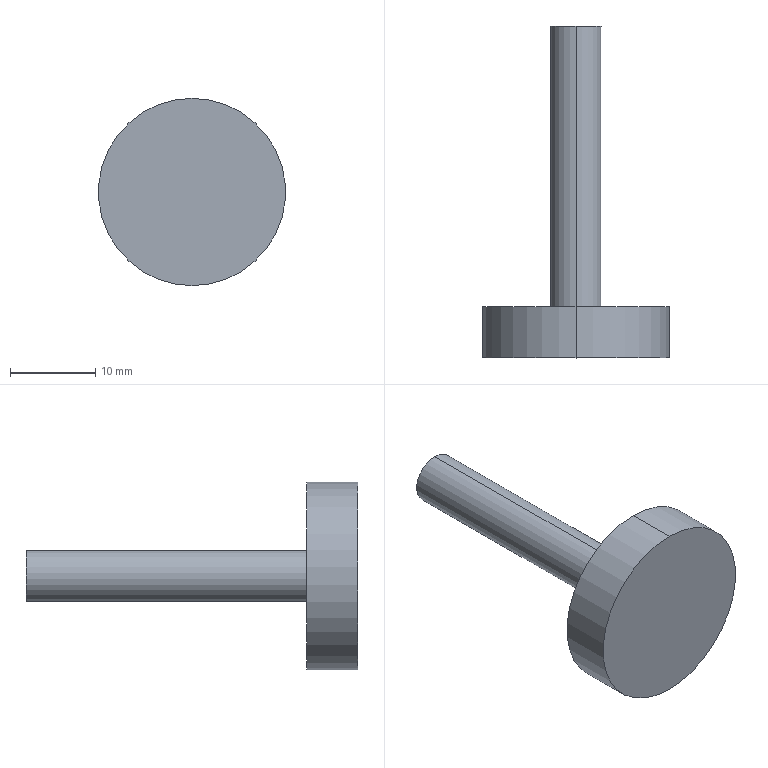Part | SolidWorks | features Extrusion 1, ICE 1 | 1 solid | 7 faces | box 22 x 39 x 22 mm | volume 3214 mm3 | cylinder 4 | plane 3 | commonest cylinder face diameters 6 x2 22 x2
STEP:
#1=CARTESIAN_POINT('',(0.,39.,3.));
#2=VERTEX_POINT('',#1);
#3=CARTESIAN_POINT('',(0.,39.,-3.));
#4=VERTEX_POINT('',#3);
#5=CARTESIAN_POINT('',(0.,39.,0.));
#6=DIRECTION('',(0.,1.,0.));
#7=DIRECTION('',(0.,0.,1.));
#8=AXIS2_PLACEMENT_3D('',#5,#6,#7);
#9=CIRCLE('',#8,3.);
#10=EDGE_CURVE('',#2,#4,#9,.T.);
#11=ORIENTED_EDGE('',*,*,#10,.F.);
#12=CARTESIAN_POINT('',(0.,6.,3.));
#13=VERTEX_POINT('',#12);
#14=CARTESIAN_POINT('',(0.,39.,3.));
#15=DIRECTION('',(0.,-1.,0.));
#16=VECTOR('',#15,1000.);
#17=LINE('',#14,#16);
#18=EDGE_CURVE('',#2,#13,#17,.T.);
#19=ORIENTED_EDGE('',*,*,#18,.T.);
#20=CARTESIAN_POINT('',(0.,6.,-3.));
#21=VERTEX_POINT('',#20);
#22=CARTESIAN_POINT('',(0.,6.,0.));
#23=DIRECTION('',(0.,1.,0.));
#24=DIRECTION('',(0.,0.,1.));
#25=AXIS2_PLACEMENT_3D('',#22,#23,#24);
#26=CIRCLE('',#25,3.);
#27=EDGE_CURVE('',#13,#21,#26,.T.);
#28=ORIENTED_EDGE('',*,*,#27,.T.);
#29=CARTESIAN_POINT('',(0.,39.,-3.));
#30=DIRECTION('',(0.,-1.,0.));
#31=VECTOR('',#30,1000.);
#32=LINE('',#29,#31);
#33=EDGE_CURVE('',#4,#21,#32,.T.);
#34=ORIENTED_EDGE('',*,*,#33,.F.);
#35=EDGE_LOOP('',(#11,#19,#28,#34));
#36=FACE_OUTER_BOUND('',#35,.T.);
#37=CARTESIAN_POINT('',(0.,39.,0.));
#38=DIRECTION('',(0.,-1.,0.));
#39=DIRECTION('',(0.,0.,-1.));
#40=AXIS2_PLACEMENT_3D('',#37,#38,#39);
#41=CYLINDRICAL_SURFACE('',#40,3.);
#42=ADVANCED_FACE('',(#36),#41,.T.);
#43=CARTESIAN_POINT('',(0.,6.,11.));
#44=VERTEX_POINT('',#43);
#45=CARTESIAN_POINT('',(0.,6.,-11.));
#46=VERTEX_POINT('',#45);
#47=CARTESIAN_POINT('',(0.,6.,0.));
#48=DIRECTION('',(0.,1.,0.));
#49=DIRECTION('',(0.,0.,1.));
#50=AXIS2_PLACEMENT_3D('',#47,#48,#49);
#51=CIRCLE('',#50,11.);
#52=EDGE_CURVE('',#44,#46,#51,.T.);
#53=ORIENTED_EDGE('',*,*,#52,.F.);
#54=CARTESIAN_POINT('',(0.,0.,11.));
#55=VERTEX_POINT('',#54);
#56=CARTESIAN_POINT('',(0.,6.,11.));
#57=DIRECTION('',(0.,-1.,0.));
#58=VECTOR('',#57,1000.);
#59=LINE('',#56,#58);
#60=EDGE_CURVE('',#44,#55,#59,.T.);
#61=ORIENTED_EDGE('',*,*,#60,.T.);
#62=CARTESIAN_POINT('',(0.,0.,-11.));
#63=VERTEX_POINT('',#62);
#64=CARTESIAN_POINT('',(0.,0.,0.));
#65=DIRECTION('',(0.,1.,0.));
#66=DIRECTION('',(0.,0.,1.));
#67=AXIS2_PLACEMENT_3D('',#64,#65,#66);
#68=CIRCLE('',#67,11.);
#69=EDGE_CURVE('',#55,#63,#68,.T.);
#70=ORIENTED_EDGE('',*,*,#69,.T.);
#71=CARTESIAN_POINT('',(0.,6.,-11.));
#72=DIRECTION('',(0.,-1.,0.));
#73=VECTOR('',#72,1000.);
#74=LINE('',#71,#73);
#75=EDGE_CURVE('',#46,#63,#74,.T.);
#76=ORIENTED_EDGE('',*,*,#75,.F.);
#77=EDGE_LOOP('',(#53,#61,#70,#76));
#78=FACE_OUTER_BOUND('',#77,.T.);
#79=CARTESIAN_POINT('',(0.,6.,0.));
#80=DIRECTION('',(0.,-1.,0.));
#81=DIRECTION('',(0.,0.,-1.));
#82=AXIS2_PLACEMENT_3D('',#79,#80,#81);
#83=CYLINDRICAL_SURFACE('',#82,11.);
#84=ADVANCED_FACE('',(#78),#83,.T.);
#85=ORIENTED_EDGE('',*,*,#60,.F.);
#86=CARTESIAN_POINT('',(0.,6.,0.));
#87=DIRECTION('',(0.,1.,0.));
#88=DIRECTION('',(0.,0.,1.));
#89=AXIS2_PLACEMENT_3D('',#86,#87,#88);
#90=CIRCLE('',#89,11.);
#91=EDGE_CURVE('',#46,#44,#90,.T.);
#92=ORIENTED_EDGE('',*,*,#91,.F.);
#93=ORIENTED_EDGE('',*,*,#75,.T.);
#94=CARTESIAN_POINT('',(0.,0.,0.));
#95=DIRECTION('',(0.,1.,0.));
#96=DIRECTION('',(0.,0.,1.));
#97=AXIS2_PLACEMENT_3D('',#94,#95,#96);
#98=CIRCLE('',#97,11.);
#99=EDGE_CURVE('',#63,#55,#98,.T.);
#100=ORIENTED_EDGE('',*,*,#99,.T.);
#101=EDGE_LOOP('',(#85,#92,#93,#100));
#102=FACE_OUTER_BOUND('',#101,.T.);
#103=CARTESIAN_POINT('',(0.,6.,0.));
#104=DIRECTION('',(0.,-1.,0.));
#105=DIRECTION('',(0.,0.,-1.));
#106=AXIS2_PLACEMENT_3D('',#103,#104,#105);
#107=CYLINDRICAL_SURFACE('',#106,11.);
#108=ADVANCED_FACE('',(#102),#107,.T.);
#109=CARTESIAN_POINT('',(0.,6.,0.));
#110=DIRECTION('',(0.,1.,0.));
#111=DIRECTION('',(0.,0.,1.));
#112=AXIS2_PLACEMENT_3D('',#109,#110,#111);
#113=CIRCLE('',#112,3.);
#114=EDGE_CURVE('',#21,#13,#113,.T.);
#115=ORIENTED_EDGE('',*,*,#114,.F.);
#116=ORIENTED_EDGE('',*,*,#27,.F.);
#117=EDGE_LOOP('',(#115,#116));
#118=FACE_BOUND('',#117,.T.);
#119=ORIENTED_EDGE('',*,*,#91,.T.);
#120=ORIENTED_EDGE('',*,*,#52,.T.);
#121=EDGE_LOOP('',(#119,#120));
#122=FACE_OUTER_BOUND('',#121,.T.);
#123=CARTESIAN_POINT('',(0.,6.,0.));
#124=DIRECTION('',(0.,1.,0.));
#125=DIRECTION('',(0.,0.,1.));
#126=AXIS2_PLACEMENT_3D('',#123,#124,#125);
#127=PLANE('',#126);
#128=ADVANCED_FACE('',(#118,#122),#127,.T.);
#129=ORIENTED_EDGE('',*,*,#99,.F.);
#130=ORIENTED_EDGE('',*,*,#69,.F.);
#131=EDGE_LOOP('',(#129,#130));
#132=FACE_OUTER_BOUND('',#131,.T.);
#133=CARTESIAN_POINT('',(0.,0.,0.));
#134=DIRECTION('',(0.,1.,0.));
#135=DIRECTION('',(0.,0.,1.));
#136=AXIS2_PLACEMENT_3D('',#133,#134,#135);
#137=PLANE('',#136);
#138=ADVANCED_FACE('',(#132),#137,.F.);
#139=ORIENTED_EDGE('',*,*,#18,.F.);
#140=CARTESIAN_POINT('',(0.,39.,0.));
#141=DIRECTION('',(0.,1.,0.));
#142=DIRECTION('',(0.,0.,1.));
#143=AXIS2_PLACEMENT_3D('',#140,#141,#142);
#144=CIRCLE('',#143,3.);
#145=EDGE_CURVE('',#4,#2,#144,.T.);
#146=ORIENTED_EDGE('',*,*,#145,.F.);
#147=ORIENTED_EDGE('',*,*,#33,.T.);
#148=ORIENTED_EDGE('',*,*,#114,.T.);
#149=EDGE_LOOP('',(#139,#146,#147,#148));
#150=FACE_OUTER_BOUND('',#149,.T.);
#151=CARTESIAN_POINT('',(0.,39.,0.));
#152=DIRECTION('',(0.,-1.,0.));
#153=DIRECTION('',(0.,0.,-1.));
#154=AXIS2_PLACEMENT_3D('',#151,#152,#153);
#155=CYLINDRICAL_SURFACE('',#154,3.);
#156=ADVANCED_FACE('',(#150),#155,.T.);
#157=ORIENTED_EDGE('',*,*,#145,.T.);
#158=ORIENTED_EDGE('',*,*,#10,.T.);
#159=EDGE_LOOP('',(#157,#158));
#160=FACE_OUTER_BOUND('',#159,.T.);
#161=CARTESIAN_POINT('',(0.,39.,0.));
#162=DIRECTION('',(0.,1.,0.));
#163=DIRECTION('',(0.,0.,1.));
#164=AXIS2_PLACEMENT_3D('',#161,#162,#163);
#165=PLANE('',#164);
#166=ADVANCED_FACE('',(#160),#165,.T.);
#167=CLOSED_SHELL('',(#42,#84,#108,#128,#138,#156,#166));
#168=MANIFOLD_SOLID_BREP('',#167);
#169=CARTESIAN_POINT('',(0.,0.,0.));
#170=DIRECTION('',(0.,0.,1.));
#171=DIRECTION('',(1.,0.,0.));
#172=AXIS2_PLACEMENT_3D('',#169,#170,#171);
#173=(LENGTH_UNIT()NAMED_UNIT(*)SI_UNIT(.MILLI.,.METRE.));
#174=UNCERTAINTY_MEASURE_WITH_UNIT(LENGTH_MEASURE(0.00001),#173,'','');
#175=(NAMED_UNIT(*)PLANE_ANGLE_UNIT()SI_UNIT($,.RADIAN.));
#176=(NAMED_UNIT(*)SI_UNIT($,.STERADIAN.)SOLID_ANGLE_UNIT());
#177=(GEOMETRIC_REPRESENTATION_CONTEXT(3)GLOBAL_UNCERTAINTY_ASSIGNED_CONTEXT((#174))GLOBAL_UNIT_ASSIGNED_CONTEXT((#173,#175,#176))REPRESENTATION_CONTEXT('',''));
#178=ADVANCED_BREP_SHAPE_REPRESENTATION('',(#168,#172),#177);